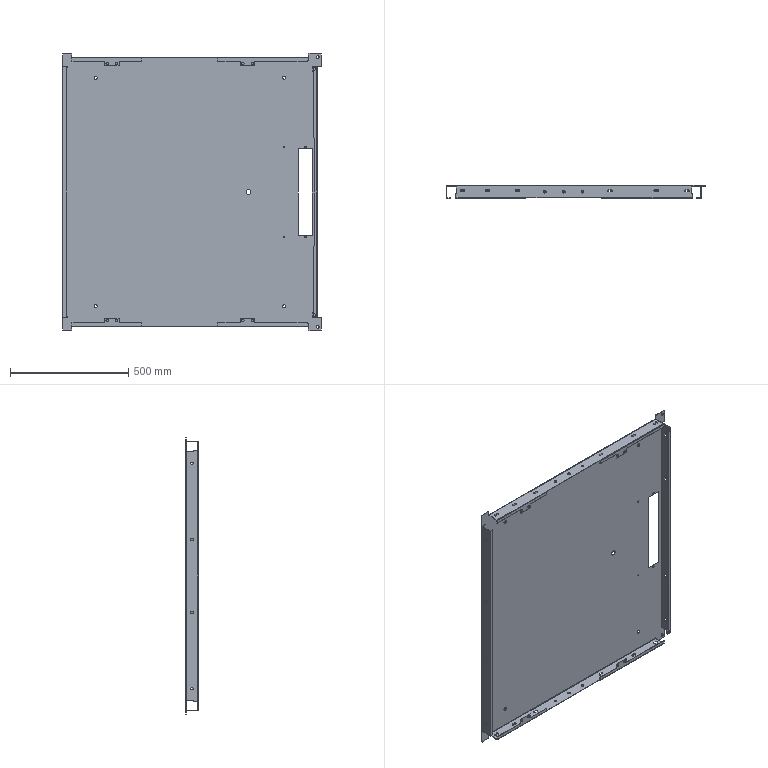Part | SolidWorks | features ICE 12, EdgeFlange 5, Fillet 5, SMBaseFlange 5, Cut 2, Chamfer 1, FlatPattern 1, MirrorPattern 1, SheetMetal 1 | 1 solid | 330 faces | box 1093 x 53 x 1171 mm | volume 2180191 mm3 | plane 186 | cylinder 144 | commonest cylinder face diameters 9 x44 10.5 x36 6 x20 10 x14 0.4 x10 3.4 x10